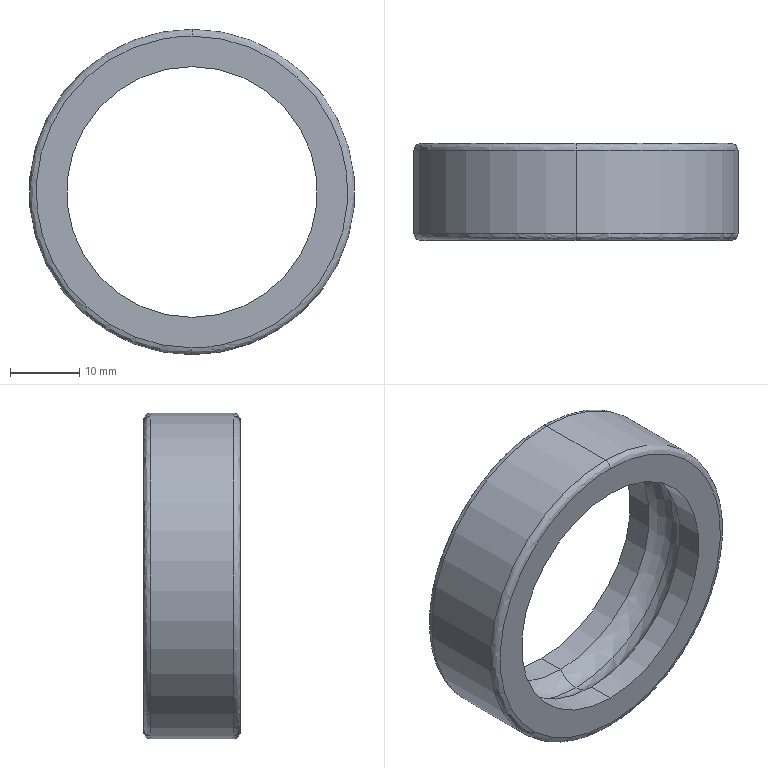Part | SolidWorks | features BaseBody 1 | 1 solid | 16 faces | box 47 x 14 x 47 mm | volume 8969 mm3 | spline 8 | cylinder 6 | plane 2 | commonest cylinder face diameters 36.2 x4 47 x2
STEP:
#1=CARTESIAN_POINT('',(0.,-7.,22.5));
#2=VERTEX_POINT('',#1);
#3=CARTESIAN_POINT('',(0.,-7.,-22.5));
#4=VERTEX_POINT('',#3);
#5=CARTESIAN_POINT('',(0.,-7.,22.5));
#6=CARTESIAN_POINT('',(45.,-7.,22.5));
#7=CARTESIAN_POINT('',(45.,-7.,-22.5));
#8=CARTESIAN_POINT('',(0.,-7.,-22.5));
#9=(BOUNDED_CURVE()B_SPLINE_CURVE(3,(#5,#6,#7,#8),.UNSPECIFIED.,.F.,.F.)B_SPLINE_CURVE_WITH_KNOTS((4,4),(0.,1.),.UNSPECIFIED.)CURVE()GEOMETRIC_REPRESENTATION_ITEM()RATIONAL_B_SPLINE_CURVE((1.,0.3333,0.3333,1.))REPRESENTATION_ITEM(''));
#10=EDGE_CURVE('',#2,#4,#9,.T.);
#11=ORIENTED_EDGE('',*,*,#10,.T.);
#12=CARTESIAN_POINT('',(0.,-6.,-23.5));
#13=VERTEX_POINT('',#12);
#14=CARTESIAN_POINT('',(0.,-6.,-22.5));
#15=DIRECTION('',(1.,0.,0.));
#16=DIRECTION('',(0.,0.,-1.));
#17=AXIS2_PLACEMENT_3D('',#14,#15,#16);
#18=CIRCLE('',#17,1.);
#19=EDGE_CURVE('',#4,#13,#18,.T.);
#20=ORIENTED_EDGE('',*,*,#19,.T.);
#21=CARTESIAN_POINT('',(0.,-6.,23.5));
#22=VERTEX_POINT('',#21);
#23=CARTESIAN_POINT('',(0.,-6.,0.));
#24=DIRECTION('',(0.,1.,0.));
#25=DIRECTION('',(0.,0.,-1.));
#26=AXIS2_PLACEMENT_3D('',#23,#24,#25);
#27=CIRCLE('',#26,23.5);
#28=EDGE_CURVE('',#22,#13,#27,.T.);
#29=ORIENTED_EDGE('',*,*,#28,.F.);
#30=CARTESIAN_POINT('',(0.,-6.,22.5));
#31=DIRECTION('',(-1.,0.,0.));
#32=DIRECTION('',(0.,0.,1.));
#33=AXIS2_PLACEMENT_3D('',#30,#31,#32);
#34=CIRCLE('',#33,1.);
#35=EDGE_CURVE('',#2,#22,#34,.T.);
#36=ORIENTED_EDGE('',*,*,#35,.F.);
#37=EDGE_LOOP('',(#11,#20,#29,#36));
#38=FACE_OUTER_BOUND('',#37,.T.);
#39=CARTESIAN_POINT('',(0.,-7.,-22.5));
#40=CARTESIAN_POINT('',(45.,-7.,-22.5));
#41=CARTESIAN_POINT('',(45.,-7.,22.5));
#42=CARTESIAN_POINT('',(0.,-7.,22.5));
#43=CARTESIAN_POINT('',(0.,-7.,-23.086));
#44=CARTESIAN_POINT('',(46.172,-7.,-23.086));
#45=CARTESIAN_POINT('',(46.172,-7.,23.086));
#46=CARTESIAN_POINT('',(0.,-7.,23.086));
#47=CARTESIAN_POINT('',(0.,-6.586,-23.5));
#48=CARTESIAN_POINT('',(47.,-6.586,-23.5));
#49=CARTESIAN_POINT('',(47.,-6.586,23.5));
#50=CARTESIAN_POINT('',(0.,-6.586,23.5));
#51=CARTESIAN_POINT('',(0.,-6.,-23.5));
#52=CARTESIAN_POINT('',(47.,-6.,-23.5));
#53=CARTESIAN_POINT('',(47.,-6.,23.5));
#54=CARTESIAN_POINT('',(0.,-6.,23.5));
#55=(BOUNDED_SURFACE()B_SPLINE_SURFACE(3,3,((#39,#40,#41,#42),(#43,#44,#45,#46),(#47,#48,#49,#50),(#51,#52,#53,#54)),.UNSPECIFIED.,.F.,.F.,.F.)B_SPLINE_SURFACE_WITH_KNOTS((4,4),(4,4),(0.,1.),(0.,1.),.UNSPECIFIED.)GEOMETRIC_REPRESENTATION_ITEM()RATIONAL_B_SPLINE_SURFACE(((1.,0.3333,0.3333,1.),(0.8047,0.2682,0.2682,0.8047),(0.8047,0.2682,0.2682,0.8047),(1.,0.3333,0.3333,1.)))REPRESENTATION_ITEM('')SURFACE());
#56=ADVANCED_FACE('',(#38),#55,.T.);
#57=CARTESIAN_POINT('',(0.,6.,-23.5));
#58=VERTEX_POINT('',#57);
#59=CARTESIAN_POINT('',(0.,6.,23.5));
#60=VERTEX_POINT('',#59);
#61=CARTESIAN_POINT('',(0.,6.,0.));
#62=DIRECTION('',(0.,-1.,0.));
#63=DIRECTION('',(0.,0.,-1.));
#64=AXIS2_PLACEMENT_3D('',#61,#62,#63);
#65=CIRCLE('',#64,23.5);
#66=EDGE_CURVE('',#58,#60,#65,.T.);
#67=ORIENTED_EDGE('',*,*,#66,.F.);
#68=CARTESIAN_POINT('',(0.,7.,-22.5));
#69=VERTEX_POINT('',#68);
#70=CARTESIAN_POINT('',(0.,6.,-22.5));
#71=DIRECTION('',(1.,0.,0.));
#72=DIRECTION('',(0.,0.,-1.));
#73=AXIS2_PLACEMENT_3D('',#70,#71,#72);
#74=CIRCLE('',#73,1.);
#75=EDGE_CURVE('',#58,#69,#74,.T.);
#76=ORIENTED_EDGE('',*,*,#75,.T.);
#77=CARTESIAN_POINT('',(0.,7.,22.5));
#78=VERTEX_POINT('',#77);
#79=CARTESIAN_POINT('',(0.,7.,-22.5));
#80=CARTESIAN_POINT('',(45.,7.,-22.5));
#81=CARTESIAN_POINT('',(45.,7.,22.5));
#82=CARTESIAN_POINT('',(0.,7.,22.5));
#83=(BOUNDED_CURVE()B_SPLINE_CURVE(3,(#79,#80,#81,#82),.UNSPECIFIED.,.F.,.T.)B_SPLINE_CURVE_WITH_KNOTS((4,4),(0.,1.),.UNSPECIFIED.)CURVE()GEOMETRIC_REPRESENTATION_ITEM()RATIONAL_B_SPLINE_CURVE((1.,0.3333,0.3333,1.))REPRESENTATION_ITEM(''));
#84=EDGE_CURVE('',#69,#78,#83,.T.);
#85=ORIENTED_EDGE('',*,*,#84,.T.);
#86=CARTESIAN_POINT('',(0.,6.,22.5));
#87=DIRECTION('',(-1.,0.,0.));
#88=DIRECTION('',(0.,0.,1.));
#89=AXIS2_PLACEMENT_3D('',#86,#87,#88);
#90=CIRCLE('',#89,1.);
#91=EDGE_CURVE('',#60,#78,#90,.T.);
#92=ORIENTED_EDGE('',*,*,#91,.F.);
#93=EDGE_LOOP('',(#67,#76,#85,#92));
#94=FACE_OUTER_BOUND('',#93,.T.);
#95=CARTESIAN_POINT('',(0.,6.,-23.5));
#96=CARTESIAN_POINT('',(47.,6.,-23.5));
#97=CARTESIAN_POINT('',(47.,6.,23.5));
#98=CARTESIAN_POINT('',(0.,6.,23.5));
#99=CARTESIAN_POINT('',(0.,6.586,-23.5));
#100=CARTESIAN_POINT('',(47.,6.586,-23.5));
#101=CARTESIAN_POINT('',(47.,6.586,23.5));
#102=CARTESIAN_POINT('',(0.,6.586,23.5));
#103=CARTESIAN_POINT('',(0.,7.,-23.086));
#104=CARTESIAN_POINT('',(46.172,7.,-23.086));
#105=CARTESIAN_POINT('',(46.172,7.,23.086));
#106=CARTESIAN_POINT('',(0.,7.,23.086));
#107=CARTESIAN_POINT('',(0.,7.,-22.5));
#108=CARTESIAN_POINT('',(45.,7.,-22.5));
#109=CARTESIAN_POINT('',(45.,7.,22.5));
#110=CARTESIAN_POINT('',(0.,7.,22.5));
#111=(BOUNDED_SURFACE()B_SPLINE_SURFACE(3,3,((#95,#96,#97,#98),(#99,#100,#101,#102),(#103,#104,#105,#106),(#107,#108,#109,#110)),.UNSPECIFIED.,.F.,.F.,.T.)B_SPLINE_SURFACE_WITH_KNOTS((4,4),(4,4),(0.,1.),(0.,1.),.UNSPECIFIED.)GEOMETRIC_REPRESENTATION_ITEM()RATIONAL_B_SPLINE_SURFACE(((1.,0.3333,0.3333,1.),(0.8047,0.2682,0.2682,0.8047),(0.8047,0.2682,0.2682,0.8047),(1.,0.3333,0.3333,1.)))REPRESENTATION_ITEM('')SURFACE());
#112=ADVANCED_FACE('',(#94),#111,.T.);
#113=CARTESIAN_POINT('',(0.,-3.107,18.1));
#114=VERTEX_POINT('',#113);
#115=CARTESIAN_POINT('',(0.,-3.107,-18.1));
#116=VERTEX_POINT('',#115);
#117=CARTESIAN_POINT('',(0.,-3.107,0.));
#118=DIRECTION('',(0.,-1.,0.));
#119=DIRECTION('',(0.,0.,-1.));
#120=AXIS2_PLACEMENT_3D('',#117,#118,#119);
#121=CIRCLE('',#120,18.1);
#122=EDGE_CURVE('',#114,#116,#121,.T.);
#123=ORIENTED_EDGE('',*,*,#122,.T.);
#124=CARTESIAN_POINT('',(0.,0.,-19.75));
#125=VERTEX_POINT('',#124);
#126=CARTESIAN_POINT('',(0.,0.,-16.));
#127=DIRECTION('',(1.,0.,0.));
#128=DIRECTION('',(0.,0.,-1.));
#129=AXIS2_PLACEMENT_3D('',#126,#127,#128);
#130=CIRCLE('',#129,3.75);
#131=EDGE_CURVE('',#116,#125,#130,.T.);
#132=ORIENTED_EDGE('',*,*,#131,.T.);
#133=CARTESIAN_POINT('',(0.,0.,19.75));
#134=VERTEX_POINT('',#133);
#135=CARTESIAN_POINT('',(0.,0.,0.));
#136=DIRECTION('',(0.,-1.,0.));
#137=DIRECTION('',(0.,0.,1.));
#138=AXIS2_PLACEMENT_3D('',#135,#136,#137);
#139=CIRCLE('',#138,19.75);
#140=EDGE_CURVE('',#134,#125,#139,.T.);
#141=ORIENTED_EDGE('',*,*,#140,.F.);
#142=CARTESIAN_POINT('',(0.,0.,16.));
#143=DIRECTION('',(-1.,0.,0.));
#144=DIRECTION('',(0.,0.,1.));
#145=AXIS2_PLACEMENT_3D('',#142,#143,#144);
#146=CIRCLE('',#145,3.75);
#147=EDGE_CURVE('',#114,#134,#146,.T.);
#148=ORIENTED_EDGE('',*,*,#147,.F.);
#149=EDGE_LOOP('',(#123,#132,#141,#148));
#150=FACE_OUTER_BOUND('',#149,.T.);
#151=CARTESIAN_POINT('',(0.,-3.107,18.1));
#152=CARTESIAN_POINT('',(-36.2,-3.107,18.1));
#153=CARTESIAN_POINT('',(-36.2,-3.107,-18.1));
#154=CARTESIAN_POINT('',(0.,-3.107,-18.1));
#155=CARTESIAN_POINT('',(0.,-2.395,19.154));
#156=CARTESIAN_POINT('',(-38.307,-2.395,19.154));
#157=CARTESIAN_POINT('',(-38.307,-2.395,-19.154));
#158=CARTESIAN_POINT('',(0.,-2.395,-19.154));
#159=CARTESIAN_POINT('',(0.,-1.272,19.75));
#160=CARTESIAN_POINT('',(-39.5,-1.272,19.75));
#161=CARTESIAN_POINT('',(-39.5,-1.272,-19.75));
#162=CARTESIAN_POINT('',(0.,-1.272,-19.75));
#163=CARTESIAN_POINT('',(0.,0.,19.75));
#164=CARTESIAN_POINT('',(-39.5,0.,19.75));
#165=CARTESIAN_POINT('',(-39.5,0.,-19.75));
#166=CARTESIAN_POINT('',(0.,0.,-19.75));
#167=(BOUNDED_SURFACE()B_SPLINE_SURFACE(3,3,((#151,#152,#153,#154),(#155,#156,#157,#158),(#159,#160,#161,#162),(#163,#164,#165,#166)),.UNSPECIFIED.,.F.,.F.,.T.)B_SPLINE_SURFACE_WITH_KNOTS((4,4),(4,4),(0.,1.),(0.,1.),.UNSPECIFIED.)GEOMETRIC_REPRESENTATION_ITEM()RATIONAL_B_SPLINE_SURFACE(((1.,0.3333,0.3333,1.),(0.9221,0.3074,0.3074,0.9221),(0.9221,0.3074,0.3074,0.9221),(1.,0.3333,0.3333,1.)))REPRESENTATION_ITEM('')SURFACE());
#168=ADVANCED_FACE('',(#150),#167,.F.);
#169=ORIENTED_EDGE('',*,*,#140,.T.);
#170=CARTESIAN_POINT('',(0.,3.107,-18.1));
#171=VERTEX_POINT('',#170);
#172=CARTESIAN_POINT('',(0.,0.,-16.));
#173=DIRECTION('',(1.,0.,0.));
#174=DIRECTION('',(0.,0.,-1.));
#175=AXIS2_PLACEMENT_3D('',#172,#173,#174);
#176=CIRCLE('',#175,3.75);
#177=EDGE_CURVE('',#125,#171,#176,.T.);
#178=ORIENTED_EDGE('',*,*,#177,.T.);
#179=CARTESIAN_POINT('',(0.,3.107,18.1));
#180=VERTEX_POINT('',#179);
#181=CARTESIAN_POINT('',(0.,3.107,0.));
#182=DIRECTION('',(0.,1.,0.));
#183=DIRECTION('',(0.,0.,-1.));
#184=AXIS2_PLACEMENT_3D('',#181,#182,#183);
#185=CIRCLE('',#184,18.1);
#186=EDGE_CURVE('',#171,#180,#185,.T.);
#187=ORIENTED_EDGE('',*,*,#186,.T.);
#188=CARTESIAN_POINT('',(0.,0.,16.));
#189=DIRECTION('',(-1.,0.,0.));
#190=DIRECTION('',(0.,0.,1.));
#191=AXIS2_PLACEMENT_3D('',#188,#189,#190);
#192=CIRCLE('',#191,3.75);
#193=EDGE_CURVE('',#134,#180,#192,.T.);
#194=ORIENTED_EDGE('',*,*,#193,.F.);
#195=EDGE_LOOP('',(#169,#178,#187,#194));
#196=FACE_OUTER_BOUND('',#195,.T.);
#197=CARTESIAN_POINT('',(0.,0.,19.75));
#198=CARTESIAN_POINT('',(-39.5,0.,19.75));
#199=CARTESIAN_POINT('',(-39.5,0.,-19.75));
#200=CARTESIAN_POINT('',(0.,0.,-19.75));
#201=CARTESIAN_POINT('',(0.,1.272,19.75));
#202=CARTESIAN_POINT('',(-39.5,1.272,19.75));
#203=CARTESIAN_POINT('',(-39.5,1.272,-19.75));
#204=CARTESIAN_POINT('',(0.,1.272,-19.75));
#205=CARTESIAN_POINT('',(0.,2.395,19.154));
#206=CARTESIAN_POINT('',(-38.307,2.395,19.154));
#207=CARTESIAN_POINT('',(-38.307,2.395,-19.154));
#208=CARTESIAN_POINT('',(0.,2.395,-19.154));
#209=CARTESIAN_POINT('',(0.,3.107,18.1));
#210=CARTESIAN_POINT('',(-36.2,3.107,18.1));
#211=CARTESIAN_POINT('',(-36.2,3.107,-18.1));
#212=CARTESIAN_POINT('',(0.,3.107,-18.1));
#213=(BOUNDED_SURFACE()B_SPLINE_SURFACE(3,3,((#197,#198,#199,#200),(#201,#202,#203,#204),(#205,#206,#207,#208),(#209,#210,#211,#212)),.UNSPECIFIED.,.F.,.F.,.F.)B_SPLINE_SURFACE_WITH_KNOTS((4,4),(4,4),(0.,1.),(0.,1.),.UNSPECIFIED.)GEOMETRIC_REPRESENTATION_ITEM()RATIONAL_B_SPLINE_SURFACE(((1.,0.3333,0.3333,1.),(0.9221,0.3074,0.3074,0.9221),(0.9221,0.3074,0.3074,0.9221),(1.,0.3333,0.3333,1.)))REPRESENTATION_ITEM('')SURFACE());
#214=ADVANCED_FACE('',(#196),#213,.F.);
#215=ORIENTED_EDGE('',*,*,#66,.T.);
#216=CARTESIAN_POINT('',(0.,7.7,23.5));
#217=DIRECTION('',(0.,-1.,0.));
#218=VECTOR('',#217,1000.);
#219=LINE('',#216,#218);
#220=EDGE_CURVE('',#60,#22,#219,.T.);
#221=ORIENTED_EDGE('',*,*,#220,.T.);
#222=ORIENTED_EDGE('',*,*,#28,.T.);
#223=CARTESIAN_POINT('',(0.,7.7,-23.5));
#224=DIRECTION('',(0.,-1.,0.));
#225=VECTOR('',#224,1000.);
#226=LINE('',#223,#225);
#227=EDGE_CURVE('',#58,#13,#226,.T.);
#228=ORIENTED_EDGE('',*,*,#227,.F.);
#229=EDGE_LOOP('',(#215,#221,#222,#228));
#230=FACE_OUTER_BOUND('',#229,.T.);
#231=CARTESIAN_POINT('',(0.,7.7,0.));
#232=DIRECTION('',(0.,-1.,0.));
#233=DIRECTION('',(0.,0.,-1.));
#234=AXIS2_PLACEMENT_3D('',#231,#232,#233);
#235=CYLINDRICAL_SURFACE('',#234,23.5);
#236=ADVANCED_FACE('',(#230),#235,.T.);
#237=ORIENTED_EDGE('',*,*,#122,.F.);
#238=CARTESIAN_POINT('',(0.,-7.,18.1));
#239=VERTEX_POINT('',#238);
#240=CARTESIAN_POINT('',(0.,7.7,18.1));
#241=DIRECTION('',(0.,-1.,0.));
#242=VECTOR('',#241,1000.);
#243=LINE('',#240,#242);
#244=EDGE_CURVE('',#114,#239,#243,.T.);
#245=ORIENTED_EDGE('',*,*,#244,.T.);
#246=CARTESIAN_POINT('',(0.,-7.,-18.1));
#247=VERTEX_POINT('',#246);
#248=CARTESIAN_POINT('',(0.,-7.,0.));
#249=DIRECTION('',(0.,1.,0.));
#250=DIRECTION('',(0.,0.,-1.));
#251=AXIS2_PLACEMENT_3D('',#248,#249,#250);
#252=CIRCLE('',#251,18.1);
#253=EDGE_CURVE('',#247,#239,#252,.T.);
#254=ORIENTED_EDGE('',*,*,#253,.F.);
#255=CARTESIAN_POINT('',(0.,7.7,-18.1));
#256=DIRECTION('',(0.,-1.,0.));
#257=VECTOR('',#256,1000.);
#258=LINE('',#255,#257);
#259=EDGE_CURVE('',#116,#247,#258,.T.);
#260=ORIENTED_EDGE('',*,*,#259,.F.);
#261=EDGE_LOOP('',(#237,#245,#254,#260));
#262=FACE_OUTER_BOUND('',#261,.T.);
#263=CARTESIAN_POINT('',(0.,7.7,0.));
#264=DIRECTION('',(0.,-1.,0.));
#265=DIRECTION('',(0.,0.,-1.));
#266=AXIS2_PLACEMENT_3D('',#263,#264,#265);
#267=CYLINDRICAL_SURFACE('',#266,18.1);
#268=ADVANCED_FACE('',(#262),#267,.F.);
#269=CARTESIAN_POINT('',(0.,7.,-18.1));
#270=VERTEX_POINT('',#269);
#271=CARTESIAN_POINT('',(0.,7.,18.1));
#272=VERTEX_POINT('',#271);
#273=CARTESIAN_POINT('',(0.,7.,0.));
#274=DIRECTION('',(0.,1.,0.));
#275=DIRECTION('',(0.,0.,-1.));
#276=AXIS2_PLACEMENT_3D('',#273,#274,#275);
#277=CIRCLE('',#276,18.1);
#278=EDGE_CURVE('',#270,#272,#277,.T.);
#279=ORIENTED_EDGE('',*,*,#278,.T.);
#280=CARTESIAN_POINT('',(0.,7.7,18.1));
#281=DIRECTION('',(0.,-1.,0.));
#282=VECTOR('',#281,1000.);
#283=LINE('',#280,#282);
#284=EDGE_CURVE('',#272,#180,#283,.T.);
#285=ORIENTED_EDGE('',*,*,#284,.T.);
#286=ORIENTED_EDGE('',*,*,#186,.F.);
#287=CARTESIAN_POINT('',(0.,7.7,-18.1));
#288=DIRECTION('',(0.,-1.,0.));
#289=VECTOR('',#288,1000.);
#290=LINE('',#287,#289);
#291=EDGE_CURVE('',#270,#171,#290,.T.);
#292=ORIENTED_EDGE('',*,*,#291,.F.);
#293=EDGE_LOOP('',(#279,#285,#286,#292));
#294=FACE_OUTER_BOUND('',#293,.T.);
#295=CARTESIAN_POINT('',(0.,7.7,0.));
#296=DIRECTION('',(0.,-1.,0.));
#297=DIRECTION('',(0.,0.,-1.));
#298=AXIS2_PLACEMENT_3D('',#295,#296,#297);
#299=CYLINDRICAL_SURFACE('',#298,18.1);
#300=ADVANCED_FACE('',(#294),#299,.F.);
#301=ORIENTED_EDGE('',*,*,#177,.F.);
#302=CARTESIAN_POINT('',(0.,0.,0.));
#303=DIRECTION('',(0.,-1.,0.));
#304=DIRECTION('',(0.,0.,1.));
#305=AXIS2_PLACEMENT_3D('',#302,#303,#304);
#306=CIRCLE('',#305,19.75);
#307=EDGE_CURVE('',#125,#134,#306,.T.);
#308=ORIENTED_EDGE('',*,*,#307,.T.);
#309=ORIENTED_EDGE('',*,*,#193,.T.);
#310=CARTESIAN_POINT('',(0.,3.107,0.));
#311=DIRECTION('',(0.,1.,0.));
#312=DIRECTION('',(0.,0.,-1.));
#313=AXIS2_PLACEMENT_3D('',#310,#311,#312);
#314=CIRCLE('',#313,18.1);
#315=EDGE_CURVE('',#180,#171,#314,.T.);
#316=ORIENTED_EDGE('',*,*,#315,.T.);
#317=EDGE_LOOP('',(#301,#308,#309,#316));
#318=FACE_OUTER_BOUND('',#317,.T.);
#319=CARTESIAN_POINT('',(0.,0.,-19.75));
#320=CARTESIAN_POINT('',(39.5,0.,-19.75));
#321=CARTESIAN_POINT('',(39.5,0.,19.75));
#322=CARTESIAN_POINT('',(0.,0.,19.75));
#323=CARTESIAN_POINT('',(0.,1.272,-19.75));
#324=CARTESIAN_POINT('',(39.5,1.272,-19.75));
#325=CARTESIAN_POINT('',(39.5,1.272,19.75));
#326=CARTESIAN_POINT('',(0.,1.272,19.75));
#327=CARTESIAN_POINT('',(0.,2.395,-19.154));
#328=CARTESIAN_POINT('',(38.307,2.395,-19.154));
#329=CARTESIAN_POINT('',(38.307,2.395,19.154));
#330=CARTESIAN_POINT('',(0.,2.395,19.154));
#331=CARTESIAN_POINT('',(0.,3.107,-18.1));
#332=CARTESIAN_POINT('',(36.2,3.107,-18.1));
#333=CARTESIAN_POINT('',(36.2,3.107,18.1));
#334=CARTESIAN_POINT('',(0.,3.107,18.1));
#335=(BOUNDED_SURFACE()B_SPLINE_SURFACE(3,3,((#319,#320,#321,#322),(#323,#324,#325,#326),(#327,#328,#329,#330),(#331,#332,#333,#334)),.UNSPECIFIED.,.F.,.F.,.T.)B_SPLINE_SURFACE_WITH_KNOTS((4,4),(4,4),(0.,1.),(0.,1.),.UNSPECIFIED.)GEOMETRIC_REPRESENTATION_ITEM()RATIONAL_B_SPLINE_SURFACE(((1.,0.3333,0.3333,1.),(0.9221,0.3074,0.3074,0.9221),(0.9221,0.3074,0.3074,0.9221),(1.,0.3333,0.3333,1.)))REPRESENTATION_ITEM('')SURFACE());
#336=ADVANCED_FACE('',(#318),#335,.F.);
#337=ORIENTED_EDGE('',*,*,#220,.F.);
#338=CARTESIAN_POINT('',(0.,6.,0.));
#339=DIRECTION('',(0.,-1.,0.));
#340=DIRECTION('',(0.,0.,-1.));
#341=AXIS2_PLACEMENT_3D('',#338,#339,#340);
#342=CIRCLE('',#341,23.5);
#343=EDGE_CURVE('',#60,#58,#342,.T.);
#344=ORIENTED_EDGE('',*,*,#343,.T.);
#345=ORIENTED_EDGE('',*,*,#227,.T.);
#346=CARTESIAN_POINT('',(0.,-6.,0.));
#347=DIRECTION('',(0.,1.,0.));
#348=DIRECTION('',(0.,0.,-1.));
#349=AXIS2_PLACEMENT_3D('',#346,#347,#348);
#350=CIRCLE('',#349,23.5);
#351=EDGE_CURVE('',#13,#22,#350,.T.);
#352=ORIENTED_EDGE('',*,*,#351,.T.);
#353=EDGE_LOOP('',(#337,#344,#345,#352));
#354=FACE_OUTER_BOUND('',#353,.T.);
#355=CARTESIAN_POINT('',(0.,7.7,0.));
#356=DIRECTION('',(0.,-1.,0.));
#357=DIRECTION('',(0.,0.,-1.));
#358=AXIS2_PLACEMENT_3D('',#355,#356,#357);
#359=CYLINDRICAL_SURFACE('',#358,23.5);
#360=ADVANCED_FACE('',(#354),#359,.T.);
#361=ORIENTED_EDGE('',*,*,#19,.F.);
#362=CARTESIAN_POINT('',(0.,-7.,-22.5));
#363=CARTESIAN_POINT('',(-45.,-7.,-22.5));
#364=CARTESIAN_POINT('',(-45.,-7.,22.5));
#365=CARTESIAN_POINT('',(0.,-7.,22.5));
#366=(BOUNDED_CURVE()B_SPLINE_CURVE(3,(#362,#363,#364,#365),.UNSPECIFIED.,.F.,.T.)B_SPLINE_CURVE_WITH_KNOTS((4,4),(0.,1.),.UNSPECIFIED.)CURVE()GEOMETRIC_REPRESENTATION_ITEM()RATIONAL_B_SPLINE_CURVE((1.,0.3333,0.3333,1.))REPRESENTATION_ITEM(''));
#367=EDGE_CURVE('',#4,#2,#366,.T.);
#368=ORIENTED_EDGE('',*,*,#367,.T.);
#369=ORIENTED_EDGE('',*,*,#35,.T.);
#370=ORIENTED_EDGE('',*,*,#351,.F.);
#371=EDGE_LOOP('',(#361,#368,#369,#370));
#372=FACE_OUTER_BOUND('',#371,.T.);
#373=CARTESIAN_POINT('',(0.,-7.,22.5));
#374=CARTESIAN_POINT('',(-45.,-7.,22.5));
#375=CARTESIAN_POINT('',(-45.,-7.,-22.5));
#376=CARTESIAN_POINT('',(0.,-7.,-22.5));
#377=CARTESIAN_POINT('',(0.,-7.,23.086));
#378=CARTESIAN_POINT('',(-46.172,-7.,23.086));
#379=CARTESIAN_POINT('',(-46.172,-7.,-23.086));
#380=CARTESIAN_POINT('',(0.,-7.,-23.086));
#381=CARTESIAN_POINT('',(0.,-6.586,23.5));
#382=CARTESIAN_POINT('',(-47.,-6.586,23.5));
#383=CARTESIAN_POINT('',(-47.,-6.586,-23.5));
#384=CARTESIAN_POINT('',(0.,-6.586,-23.5));
#385=CARTESIAN_POINT('',(0.,-6.,23.5));
#386=CARTESIAN_POINT('',(-47.,-6.,23.5));
#387=CARTESIAN_POINT('',(-47.,-6.,-23.5));
#388=CARTESIAN_POINT('',(0.,-6.,-23.5));
#389=(BOUNDED_SURFACE()B_SPLINE_SURFACE(3,3,((#373,#374,#375,#376),(#377,#378,#379,#380),(#381,#382,#383,#384),(#385,#386,#387,#388)),.UNSPECIFIED.,.F.,.F.,.T.)B_SPLINE_SURFACE_WITH_KNOTS((4,4),(4,4),(0.,1.),(0.,1.),.UNSPECIFIED.)GEOMETRIC_REPRESENTATION_ITEM()RATIONAL_B_SPLINE_SURFACE(((1.,0.3333,0.3333,1.),(0.8047,0.2682,0.2682,0.8047),(0.8047,0.2682,0.2682,0.8047),(1.,0.3333,0.3333,1.)))REPRESENTATION_ITEM('')SURFACE());
#390=ADVANCED_FACE('',(#372),#389,.T.);
#391=ORIENTED_EDGE('',*,*,#75,.F.);
#392=ORIENTED_EDGE('',*,*,#343,.F.);
#393=ORIENTED_EDGE('',*,*,#91,.T.);
#394=CARTESIAN_POINT('',(0.,7.,22.5));
#395=CARTESIAN_POINT('',(-45.,7.,22.5));
#396=CARTESIAN_POINT('',(-45.,7.,-22.5));
#397=CARTESIAN_POINT('',(0.,7.,-22.5));
#398=(BOUNDED_CURVE()B_SPLINE_CURVE(3,(#394,#395,#396,#397),.UNSPECIFIED.,.F.,.T.)B_SPLINE_CURVE_WITH_KNOTS((4,4),(0.,1.),.UNSPECIFIED.)CURVE()GEOMETRIC_REPRESENTATION_ITEM()RATIONAL_B_SPLINE_CURVE((1.,0.3333,0.3333,1.))REPRESENTATION_ITEM(''));
#399=EDGE_CURVE('',#78,#69,#398,.T.);
#400=ORIENTED_EDGE('',*,*,#399,.T.);
#401=EDGE_LOOP('',(#391,#392,#393,#400));
#402=FACE_OUTER_BOUND('',#401,.T.);
#403=CARTESIAN_POINT('',(0.,6.,23.5));
#404=CARTESIAN_POINT('',(-47.,6.,23.5));
#405=CARTESIAN_POINT('',(-47.,6.,-23.5));
#406=CARTESIAN_POINT('',(0.,6.,-23.5));
#407=CARTESIAN_POINT('',(0.,6.586,23.5));
#408=CARTESIAN_POINT('',(-47.,6.586,23.5));
#409=CARTESIAN_POINT('',(-47.,6.586,-23.5));
#410=CARTESIAN_POINT('',(0.,6.586,-23.5));
#411=CARTESIAN_POINT('',(0.,7.,23.086));
#412=CARTESIAN_POINT('',(-46.172,7.,23.086));
#413=CARTESIAN_POINT('',(-46.172,7.,-23.086));
#414=CARTESIAN_POINT('',(0.,7.,-23.086));
#415=CARTESIAN_POINT('',(0.,7.,22.5));
#416=CARTESIAN_POINT('',(-45.,7.,22.5));
#417=CARTESIAN_POINT('',(-45.,7.,-22.5));
#418=CARTESIAN_POINT('',(0.,7.,-22.5));
#419=(BOUNDED_SURFACE()B_SPLINE_SURFACE(3,3,((#403,#404,#405,#406),(#407,#408,#409,#410),(#411,#412,#413,#414),(#415,#416,#417,#418)),.UNSPECIFIED.,.F.,.F.,.F.)B_SPLINE_SURFACE_WITH_KNOTS((4,4),(4,4),(0.,1.),(0.,1.),.UNSPECIFIED.)GEOMETRIC_REPRESENTATION_ITEM()RATIONAL_B_SPLINE_SURFACE(((1.,0.3333,0.3333,1.),(0.8047,0.2682,0.2682,0.8047),(0.8047,0.2682,0.2682,0.8047),(1.,0.3333,0.3333,1.)))REPRESENTATION_ITEM('')SURFACE());
#420=ADVANCED_FACE('',(#402),#419,.T.);
#421=ORIENTED_EDGE('',*,*,#253,.T.);
#422=CARTESIAN_POINT('',(0.,-7.,0.));
#423=DIRECTION('',(0.,1.,0.));
#424=DIRECTION('',(0.,0.,-1.));
#425=AXIS2_PLACEMENT_3D('',#422,#423,#424);
#426=CIRCLE('',#425,18.1);
#427=EDGE_CURVE('',#239,#247,#426,.T.);
#428=ORIENTED_EDGE('',*,*,#427,.T.);
#429=EDGE_LOOP('',(#421,#428));
#430=FACE_BOUND('',#429,.T.);
#431=ORIENTED_EDGE('',*,*,#367,.F.);
#432=ORIENTED_EDGE('',*,*,#10,.F.);
#433=EDGE_LOOP('',(#431,#432));
#434=FACE_OUTER_BOUND('',#433,.T.);
#435=CARTESIAN_POINT('',(0.,-7.,0.));
#436=DIRECTION('',(0.,-1.,0.));
#437=DIRECTION('',(0.,0.,-1.));
#438=AXIS2_PLACEMENT_3D('',#435,#436,#437);
#439=PLANE('',#438);
#440=ADVANCED_FACE('',(#430,#434),#439,.T.);
#441=ORIENTED_EDGE('',*,*,#278,.F.);
#442=CARTESIAN_POINT('',(0.,7.,0.));
#443=DIRECTION('',(0.,1.,0.));
#444=DIRECTION('',(0.,0.,-1.));
#445=AXIS2_PLACEMENT_3D('',#442,#443,#444);
#446=CIRCLE('',#445,18.1);
#447=EDGE_CURVE('',#272,#270,#446,.T.);
#448=ORIENTED_EDGE('',*,*,#447,.F.);
#449=EDGE_LOOP('',(#441,#448));
#450=FACE_BOUND('',#449,.T.);
#451=ORIENTED_EDGE('',*,*,#399,.F.);
#452=ORIENTED_EDGE('',*,*,#84,.F.);
#453=EDGE_LOOP('',(#451,#452));
#454=FACE_OUTER_BOUND('',#453,.T.);
#455=CARTESIAN_POINT('',(0.,7.,0.));
#456=DIRECTION('',(0.,-1.,0.));
#457=DIRECTION('',(0.,0.,-1.));
#458=AXIS2_PLACEMENT_3D('',#455,#456,#457);
#459=PLANE('',#458);
#460=ADVANCED_FACE('',(#450,#454),#459,.F.);
#461=ORIENTED_EDGE('',*,*,#244,.F.);
#462=CARTESIAN_POINT('',(0.,-3.107,0.));
#463=DIRECTION('',(0.,-1.,0.));
#464=DIRECTION('',(0.,0.,-1.));
#465=AXIS2_PLACEMENT_3D('',#462,#463,#464);
#466=CIRCLE('',#465,18.1);
#467=EDGE_CURVE('',#116,#114,#466,.T.);
#468=ORIENTED_EDGE('',*,*,#467,.F.);
#469=ORIENTED_EDGE('',*,*,#259,.T.);
#470=ORIENTED_EDGE('',*,*,#427,.F.);
#471=EDGE_LOOP('',(#461,#468,#469,#470));
#472=FACE_OUTER_BOUND('',#471,.T.);
#473=CARTESIAN_POINT('',(0.,7.7,0.));
#474=DIRECTION('',(0.,-1.,0.));
#475=DIRECTION('',(0.,0.,-1.));
#476=AXIS2_PLACEMENT_3D('',#473,#474,#475);
#477=CYLINDRICAL_SURFACE('',#476,18.1);
#478=ADVANCED_FACE('',(#472),#477,.F.);
#479=ORIENTED_EDGE('',*,*,#284,.F.);
#480=ORIENTED_EDGE('',*,*,#447,.T.);
#481=ORIENTED_EDGE('',*,*,#291,.T.);
#482=ORIENTED_EDGE('',*,*,#315,.F.);
#483=EDGE_LOOP('',(#479,#480,#481,#482));
#484=FACE_OUTER_BOUND('',#483,.T.);
#485=CARTESIAN_POINT('',(0.,7.7,0.));
#486=DIRECTION('',(0.,-1.,0.));
#487=DIRECTION('',(0.,0.,-1.));
#488=AXIS2_PLACEMENT_3D('',#485,#486,#487);
#489=CYLINDRICAL_SURFACE('',#488,18.1);
#490=ADVANCED_FACE('',(#484),#489,.F.);
#491=ORIENTED_EDGE('',*,*,#131,.F.);
#492=ORIENTED_EDGE('',*,*,#467,.T.);
#493=ORIENTED_EDGE('',*,*,#147,.T.);
#494=ORIENTED_EDGE('',*,*,#307,.F.);
#495=EDGE_LOOP('',(#491,#492,#493,#494));
#496=FACE_OUTER_BOUND('',#495,.T.);
#497=CARTESIAN_POINT('',(0.,-3.107,-18.1));
#498=CARTESIAN_POINT('',(36.2,-3.107,-18.1));
#499=CARTESIAN_POINT('',(36.2,-3.107,18.1));
#500=CARTESIAN_POINT('',(0.,-3.107,18.1));
#501=CARTESIAN_POINT('',(0.,-2.395,-19.154));
#502=CARTESIAN_POINT('',(38.307,-2.395,-19.154));
#503=CARTESIAN_POINT('',(38.307,-2.395,19.154));
#504=CARTESIAN_POINT('',(0.,-2.395,19.154));
#505=CARTESIAN_POINT('',(0.,-1.272,-19.75));
#506=CARTESIAN_POINT('',(39.5,-1.272,-19.75));
#507=CARTESIAN_POINT('',(39.5,-1.272,19.75));
#508=CARTESIAN_POINT('',(0.,-1.272,19.75));
#509=CARTESIAN_POINT('',(0.,0.,-19.75));
#510=CARTESIAN_POINT('',(39.5,0.,-19.75));
#511=CARTESIAN_POINT('',(39.5,0.,19.75));
#512=CARTESIAN_POINT('',(0.,0.,19.75));
#513=(BOUNDED_SURFACE()B_SPLINE_SURFACE(3,3,((#497,#498,#499,#500),(#501,#502,#503,#504),(#505,#506,#507,#508),(#509,#510,#511,#512)),.UNSPECIFIED.,.F.,.F.,.F.)B_SPLINE_SURFACE_WITH_KNOTS((4,4),(4,4),(0.,1.),(0.,1.),.UNSPECIFIED.)GEOMETRIC_REPRESENTATION_ITEM()RATIONAL_B_SPLINE_SURFACE(((1.,0.3333,0.3333,1.),(0.9221,0.3074,0.3074,0.9221),(0.9221,0.3074,0.3074,0.9221),(1.,0.3333,0.3333,1.)))REPRESENTATION_ITEM('')SURFACE());
#514=ADVANCED_FACE('',(#496),#513,.F.);
#515=CLOSED_SHELL('',(#56,#112,#168,#214,#236,#268,#300,#336,#360,#390,#420,#440,#460,#478,#490,#514));
#516=MANIFOLD_SOLID_BREP('',#515);
#517=CARTESIAN_POINT('',(0.,0.,0.));
#518=DIRECTION('',(0.,0.,1.));
#519=DIRECTION('',(1.,0.,0.));
#520=AXIS2_PLACEMENT_3D('',#517,#518,#519);
#521=(LENGTH_UNIT()NAMED_UNIT(*)SI_UNIT(.MILLI.,.METRE.));
#522=UNCERTAINTY_MEASURE_WITH_UNIT(LENGTH_MEASURE(0.00001),#521,'','');
#523=(NAMED_UNIT(*)PLANE_ANGLE_UNIT()SI_UNIT($,.RADIAN.));
#524=(NAMED_UNIT(*)SI_UNIT($,.STERADIAN.)SOLID_ANGLE_UNIT());
#525=(GEOMETRIC_REPRESENTATION_CONTEXT(3)GLOBAL_UNCERTAINTY_ASSIGNED_CONTEXT((#522))GLOBAL_UNIT_ASSIGNED_CONTEXT((#521,#523,#524))REPRESENTATION_CONTEXT('',''));
#526=ADVANCED_BREP_SHAPE_REPRESENTATION('',(#516,#520),#525);